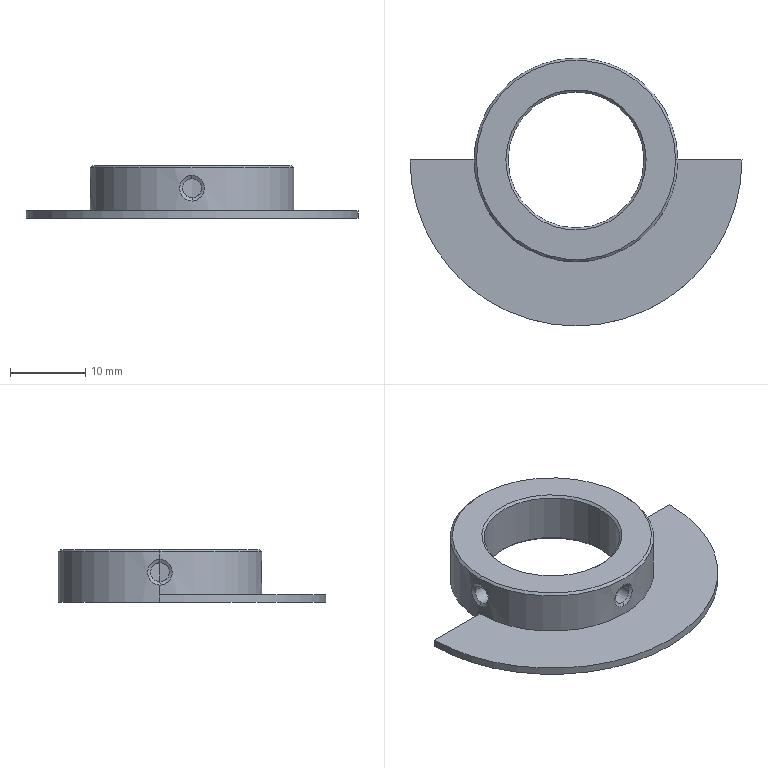Part | NX | 1 solid | 24 faces | box 44 x 35.5 x 7 mm | volume 2646 mm3 | cylinder 9 | cone 6 | plane 5 | spline 4 | commonest cylinder face diameters 2.5 x4 18 x2 27 x2 44 x1
STEP:
#1=CARTESIAN_POINT('',(-13.2,0.,7.));
#2=VERTEX_POINT('',#1);
#3=CARTESIAN_POINT('',(13.2,0.,7.));
#4=VERTEX_POINT('',#3);
#5=CARTESIAN_POINT('',(0.,0.,7.));
#6=DIRECTION('',(0.,0.,-1.));
#7=DIRECTION('',(-1.,0.,0.));
#8=AXIS2_PLACEMENT_3D('',#5,#6,#7);
#9=CIRCLE('',#8,13.2);
#10=EDGE_CURVE('',#2,#4,#9,.T.);
#11=ORIENTED_EDGE('',*,*,#10,.F.);
#12=CARTESIAN_POINT('',(0.,0.,7.));
#13=DIRECTION('',(0.,0.,-1.));
#14=DIRECTION('',(-1.,0.,0.));
#15=AXIS2_PLACEMENT_3D('',#12,#13,#14);
#16=CIRCLE('',#15,13.2);
#17=EDGE_CURVE('',#4,#2,#16,.T.);
#18=ORIENTED_EDGE('',*,*,#17,.F.);
#19=EDGE_LOOP('',(#11,#18));
#20=FACE_BOUND('',#19,.T.);
#21=CARTESIAN_POINT('',(9.3,0.,7.));
#22=VERTEX_POINT('',#21);
#23=CARTESIAN_POINT('',(-9.3,0.,7.));
#24=VERTEX_POINT('',#23);
#25=CARTESIAN_POINT('',(0.,0.,7.));
#26=DIRECTION('',(0.,0.,1.));
#27=DIRECTION('',(1.,0.,0.));
#28=AXIS2_PLACEMENT_3D('',#25,#26,#27);
#29=CIRCLE('',#28,9.3);
#30=EDGE_CURVE('',#22,#24,#29,.T.);
#31=ORIENTED_EDGE('',*,*,#30,.F.);
#32=CARTESIAN_POINT('',(0.,0.,7.));
#33=DIRECTION('',(0.,0.,1.));
#34=DIRECTION('',(1.,0.,0.));
#35=AXIS2_PLACEMENT_3D('',#32,#33,#34);
#36=CIRCLE('',#35,9.3);
#37=EDGE_CURVE('',#24,#22,#36,.T.);
#38=ORIENTED_EDGE('',*,*,#37,.F.);
#39=EDGE_LOOP('',(#31,#38));
#40=FACE_BOUND('',#39,.T.);
#41=CARTESIAN_POINT('',(0.,0.,7.));
#42=DIRECTION('',(0.,0.,1.));
#43=DIRECTION('',(1.,0.,0.));
#44=AXIS2_PLACEMENT_3D('',#41,#42,#43);
#45=PLANE('',#44);
#46=ADVANCED_FACE('',(#20,#40),#45,.T.);
#47=CARTESIAN_POINT('',(13.5,0.,6.7));
#48=VERTEX_POINT('',#47);
#49=CARTESIAN_POINT('',(-13.5,0.,6.7));
#50=VERTEX_POINT('',#49);
#51=CARTESIAN_POINT('',(0.,0.,6.7));
#52=DIRECTION('',(0.,0.,-1.));
#53=DIRECTION('',(-1.,0.,0.));
#54=AXIS2_PLACEMENT_3D('',#51,#52,#53);
#55=CIRCLE('',#54,13.5);
#56=EDGE_CURVE('',#48,#50,#55,.T.);
#57=ORIENTED_EDGE('',*,*,#56,.T.);
#58=CARTESIAN_POINT('',(-13.5,0.,5.7));
#59=VERTEX_POINT('',#58);
#60=CARTESIAN_POINT('',(-13.5,0.,0.));
#61=DIRECTION('',(0.,0.,1.));
#62=VECTOR('',#61,1000.);
#63=LINE('',#60,#62);
#64=EDGE_CURVE('',#50,#59,#63,.F.);
#65=ORIENTED_EDGE('',*,*,#64,.T.);
#66=CARTESIAN_POINT('',(-13.5,-0.01105,2.3));
#67=VERTEX_POINT('',#66);
#68=CARTESIAN_POINT('',(-13.5,0.,5.7));
#69=CARTESIAN_POINT('',(-13.5,-0.4479,5.699));
#70=CARTESIAN_POINT('',(-13.448,-1.303,5.293));
#71=CARTESIAN_POINT('',(-13.378,-1.79,4.006));
#72=CARTESIAN_POINT('',(-13.446,-1.314,2.718));
#73=CARTESIAN_POINT('',(-13.5,-0.4559,2.303));
#74=CARTESIAN_POINT('',(-13.5,-0.01105,2.3));
#75=B_SPLINE_CURVE_WITH_KNOTS('',3,(#68,#69,#70,#71,#72,#73,#74),.UNSPECIFIED.,.F.,.F.,(4,1,1,1,4),(0.,0.25,0.5,0.75,1.),.UNSPECIFIED.);
#76=EDGE_CURVE('',#67,#59,#75,.F.);
#77=ORIENTED_EDGE('',*,*,#76,.F.);
#78=CARTESIAN_POINT('',(-13.5,0.,2.3));
#79=VERTEX_POINT('',#78);
#80=CARTESIAN_POINT('',(-13.5,0.,2.3));
#81=CARTESIAN_POINT('',(-13.5,-0.003678,2.3));
#82=CARTESIAN_POINT('',(-13.5,-0.007364,2.3));
#83=CARTESIAN_POINT('',(-13.5,-0.01105,2.3));
#84=B_SPLINE_CURVE_WITH_KNOTS('',3,(#80,#81,#82,#83),.UNSPECIFIED.,.F.,.F.,(4,4),(9.217,9.227),.UNSPECIFIED.);
#85=EDGE_CURVE('',#79,#67,#84,.T.);
#86=ORIENTED_EDGE('',*,*,#85,.F.);
#87=CARTESIAN_POINT('',(-13.5,0.,1.));
#88=VERTEX_POINT('',#87);
#89=CARTESIAN_POINT('',(-13.5,0.,0.));
#90=DIRECTION('',(0.,0.,1.));
#91=VECTOR('',#90,1000.);
#92=LINE('',#89,#91);
#93=EDGE_CURVE('',#88,#79,#92,.T.);
#94=ORIENTED_EDGE('',*,*,#93,.F.);
#95=CARTESIAN_POINT('',(13.5,0.,1.));
#96=VERTEX_POINT('',#95);
#97=CARTESIAN_POINT('',(0.,0.,1.));
#98=DIRECTION('',(0.,0.,1.));
#99=DIRECTION('',(1.,0.,0.));
#100=AXIS2_PLACEMENT_3D('',#97,#98,#99);
#101=CIRCLE('',#100,13.5);
#102=EDGE_CURVE('',#88,#96,#101,.T.);
#103=ORIENTED_EDGE('',*,*,#102,.T.);
#104=CARTESIAN_POINT('',(13.5,0.,0.));
#105=DIRECTION('',(0.,0.,1.));
#106=VECTOR('',#105,1000.);
#107=LINE('',#104,#106);
#108=EDGE_CURVE('',#48,#96,#107,.F.);
#109=ORIENTED_EDGE('',*,*,#108,.F.);
#110=EDGE_LOOP('',(#57,#65,#77,#86,#94,#103,#109));
#111=FACE_BOUND('',#110,.T.);
#112=CARTESIAN_POINT('',(-0.01314,-13.5,5.7));
#113=VERTEX_POINT('',#112);
#114=CARTESIAN_POINT('',(0.01305,-13.5,2.3));
#115=VERTEX_POINT('',#114);
#116=CARTESIAN_POINT('',(0.01305,-13.5,2.3));
#117=CARTESIAN_POINT('',(-0.4359,-13.5,2.297));
#118=CARTESIAN_POINT('',(-1.296,-13.449,2.698));
#119=CARTESIAN_POINT('',(-1.791,-13.378,3.986));
#120=CARTESIAN_POINT('',(-1.318,-13.446,5.278));
#121=CARTESIAN_POINT('',(-0.4589,-13.5,5.696));
#122=CARTESIAN_POINT('',(-0.01314,-13.5,5.7));
#123=B_SPLINE_CURVE_WITH_KNOTS('',3,(#116,#117,#118,#119,#120,#121,#122),.UNSPECIFIED.,.F.,.F.,(4,1,1,1,4),(0.,0.25,0.5,0.75,1.),.UNSPECIFIED.);
#124=EDGE_CURVE('',#113,#115,#123,.F.);
#125=ORIENTED_EDGE('',*,*,#124,.F.);
#126=CARTESIAN_POINT('',(-0.01314,-13.5,5.7));
#127=CARTESIAN_POINT('',(0.4307,-13.5,5.704));
#128=CARTESIAN_POINT('',(1.299,-13.448,5.302));
#129=CARTESIAN_POINT('',(1.79,-13.378,4.012));
#130=CARTESIAN_POINT('',(1.317,-13.446,2.721));
#131=CARTESIAN_POINT('',(0.4589,-13.5,2.304));
#132=CARTESIAN_POINT('',(0.01305,-13.5,2.3));
#133=B_SPLINE_CURVE_WITH_KNOTS('',3,(#126,#127,#128,#129,#130,#131,#132),.UNSPECIFIED.,.F.,.F.,(4,1,1,1,4),(0.,0.25,0.5,0.75,1.),.UNSPECIFIED.);
#134=EDGE_CURVE('',#115,#113,#133,.F.);
#135=ORIENTED_EDGE('',*,*,#134,.F.);
#136=EDGE_LOOP('',(#125,#135));
#137=FACE_BOUND('',#136,.T.);
#138=CARTESIAN_POINT('',(0.,0.,0.));
#139=DIRECTION('',(0.,0.,1.));
#140=DIRECTION('',(1.,0.,0.));
#141=AXIS2_PLACEMENT_3D('',#138,#139,#140);
#142=CYLINDRICAL_SURFACE('',#141,13.5);
#143=ADVANCED_FACE('',(#111,#137),#142,.T.);
#144=ORIENTED_EDGE('',*,*,#124,.T.);
#145=CARTESIAN_POINT('',(0.009148,-13.24,2.75));
#146=VERTEX_POINT('',#145);
#147=CARTESIAN_POINT('',(0.009148,-13.24,2.75));
#148=CARTESIAN_POINT('',(0.01305,-13.5,2.3));
#149=B_SPLINE_CURVE_WITH_KNOTS('',1,(#147,#148),.UNSPECIFIED.,.F.,.F.,(2,2),(0.,1.),.UNSPECIFIED.);
#150=EDGE_CURVE('',#146,#115,#149,.T.);
#151=ORIENTED_EDGE('',*,*,#150,.F.);
#152=CARTESIAN_POINT('',(-0.0007957,-13.24,2.75));
#153=VERTEX_POINT('',#152);
#154=CARTESIAN_POINT('',(-0.0007956,-13.24,2.75));
#155=CARTESIAN_POINT('',(0.002519,-13.24,2.75));
#156=CARTESIAN_POINT('',(0.005833,-13.24,2.75));
#157=CARTESIAN_POINT('',(0.009147,-13.24,2.75));
#158=B_SPLINE_CURVE_WITH_KNOTS('',3,(#154,#155,#156,#157),.UNSPECIFIED.,.F.,.F.,(4,4),(0.,1.),.UNSPECIFIED.);
#159=EDGE_CURVE('',#153,#146,#158,.T.);
#160=ORIENTED_EDGE('',*,*,#159,.F.);
#161=CARTESIAN_POINT('',(-1.25,-13.182,4.));
#162=VERTEX_POINT('',#161);
#163=CARTESIAN_POINT('',(-1.25,-13.182,4.));
#164=CARTESIAN_POINT('',(-1.25,-13.182,3.841));
#165=CARTESIAN_POINT('',(-1.18,-13.188,3.551));
#166=CARTESIAN_POINT('',(-1.073,-13.198,3.345));
#167=CARTESIAN_POINT('',(-0.8867,-13.211,3.097));
#168=CARTESIAN_POINT('',(-0.6376,-13.225,2.917));
#169=CARTESIAN_POINT('',(-0.4359,-13.234,2.816));
#170=CARTESIAN_POINT('',(-0.1547,-13.24,2.75));
#171=CARTESIAN_POINT('',(-0.0007956,-13.24,2.75));
#172=B_SPLINE_CURVE_WITH_KNOTS('',3,(#163,#164,#165,#166,#167,#168,#169,#170,#171),.UNSPECIFIED.,.F.,.F.,(4,1,1,1,1,1,4),(0.,0.25,0.375,0.5,0.625,0.75,1.),.UNSPECIFIED.);
#173=EDGE_CURVE('',#162,#153,#172,.T.);
#174=ORIENTED_EDGE('',*,*,#173,.F.);
#175=CARTESIAN_POINT('',(-0.009525,-13.24,5.25));
#176=VERTEX_POINT('',#175);
#177=CARTESIAN_POINT('',(-0.009525,-13.24,5.25));
#178=CARTESIAN_POINT('',(-0.1614,-13.24,5.249));
#179=CARTESIAN_POINT('',(-0.4452,-13.234,5.18));
#180=CARTESIAN_POINT('',(-0.6425,-13.225,5.08));
#181=CARTESIAN_POINT('',(-0.891,-13.211,4.899));
#182=CARTESIAN_POINT('',(-1.074,-13.198,4.653));
#183=CARTESIAN_POINT('',(-1.181,-13.188,4.446));
#184=CARTESIAN_POINT('',(-1.25,-13.182,4.158));
#185=CARTESIAN_POINT('',(-1.25,-13.182,4.));
#186=B_SPLINE_CURVE_WITH_KNOTS('',3,(#177,#178,#179,#180,#181,#182,#183,#184,#185),.UNSPECIFIED.,.F.,.F.,(4,1,1,1,1,1,4),(0.,0.25,0.375,0.5,0.625,0.75,1.),.UNSPECIFIED.);
#187=EDGE_CURVE('',#176,#162,#186,.T.);
#188=ORIENTED_EDGE('',*,*,#187,.F.);
#189=CARTESIAN_POINT('',(-0.009525,-13.24,5.25));
#190=CARTESIAN_POINT('',(-0.01314,-13.5,5.7));
#191=B_SPLINE_CURVE_WITH_KNOTS('',1,(#189,#190),.UNSPECIFIED.,.F.,.F.,(2,2),(0.,1.),.UNSPECIFIED.);
#192=EDGE_CURVE('',#176,#113,#191,.T.);
#193=ORIENTED_EDGE('',*,*,#192,.T.);
#194=EDGE_LOOP('',(#144,#151,#160,#174,#188,#193));
#195=FACE_BOUND('',#194,.T.);
#196=CARTESIAN_POINT('',(-0.009525,-13.24,5.25));
#197=CARTESIAN_POINT('',(-0.01314,-13.5,5.7));
#198=CARTESIAN_POINT('',(-0.01524,-13.24,5.25));
#199=CARTESIAN_POINT('',(-0.02103,-13.5,5.7));
#200=CARTESIAN_POINT('',(-0.02096,-13.24,5.25));
#201=CARTESIAN_POINT('',(-0.02892,-13.5,5.7));
#202=CARTESIAN_POINT('',(-0.05049,-13.24,5.249));
#203=CARTESIAN_POINT('',(-0.06965,-13.5,5.699));
#204=CARTESIAN_POINT('',(-0.07427,-13.24,5.248));
#205=CARTESIAN_POINT('',(-0.1025,-13.5,5.697));
#206=CARTESIAN_POINT('',(-0.1973,-13.239,5.238));
#207=CARTESIAN_POINT('',(-0.2718,-13.498,5.682));
#208=CARTESIAN_POINT('',(-0.295,-13.237,5.219));
#209=CARTESIAN_POINT('',(-0.4066,-13.494,5.652));
#210=CARTESIAN_POINT('',(-0.586,-13.229,5.123));
#211=CARTESIAN_POINT('',(-0.7985,-13.479,5.509));
#212=CARTESIAN_POINT('',(-0.7633,-13.219,5.012));
#213=CARTESIAN_POINT('',(-1.031,-13.462,5.344));
#214=CARTESIAN_POINT('',(-1.05,-13.2,4.71));
#215=CARTESIAN_POINT('',(-1.391,-13.429,4.925));
#216=CARTESIAN_POINT('',(-1.154,-13.191,4.524));
#217=CARTESIAN_POINT('',(-1.516,-13.415,4.679));
#218=CARTESIAN_POINT('',(-1.262,-13.181,4.118));
#219=CARTESIAN_POINT('',(-1.644,-13.4,4.15));
#220=CARTESIAN_POINT('',(-1.264,-13.181,3.902));
#221=CARTESIAN_POINT('',(-1.646,-13.399,3.876));
#222=CARTESIAN_POINT('',(-1.162,-13.19,3.492));
#223=CARTESIAN_POINT('',(-1.525,-13.414,3.342));
#224=CARTESIAN_POINT('',(-1.058,-13.199,3.303));
#225=CARTESIAN_POINT('',(-1.402,-13.428,3.092));
#226=CARTESIAN_POINT('',(-0.7739,-13.218,2.996));
#227=CARTESIAN_POINT('',(-1.044,-13.461,2.668));
#228=CARTESIAN_POINT('',(-0.5977,-13.228,2.883));
#229=CARTESIAN_POINT('',(-0.8144,-13.478,2.501));
#230=CARTESIAN_POINT('',(-0.269,-13.238,2.771));
#231=CARTESIAN_POINT('',(-0.3717,-13.496,2.333));
#232=CARTESIAN_POINT('',(-0.1303,-13.24,2.749));
#233=CARTESIAN_POINT('',(-0.1794,-13.5,2.299));
#234=CARTESIAN_POINT('',(0.009148,-13.24,2.75));
#235=CARTESIAN_POINT('',(0.01305,-13.5,2.3));
#236=CARTESIAN_POINT('',(0.009386,-13.24,2.75));
#237=CARTESIAN_POINT('',(0.01338,-13.5,2.3));
#238=CARTESIAN_POINT('',(0.009623,-13.24,2.75));
#239=CARTESIAN_POINT('',(0.01371,-13.5,2.3));
#240=CARTESIAN_POINT('',(0.009861,-13.24,2.75));
#241=CARTESIAN_POINT('',(0.01404,-13.5,2.3));
#242=B_SPLINE_SURFACE_WITH_KNOTS('',3,1,((#196,#197),(#198,#199),(#200,#201),(#202,#203),(#204,#205),(#206,#207),(#208,#209),(#210,#211),(#212,#213),(#214,#215),(#216,#217),(#218,#219),(#220,#221),(#222,#223),(#224,#225),(#226,#227),(#228,#229),(#230,#231),(#232,#233),(#234,#235),(#236,#237),(#238,#239),(#240,#241)),.RULED_SURF.,.F.,.F.,.F.,(4,2,2,2,2,2,2,2,2,3,4),(2,2),(0.,0.02041,0.1054,0.4606,1.192,1.919,2.647,3.381,4.112,4.613,4.614),(0.,1.),.UNSPECIFIED.);
#243=ADVANCED_FACE('',(#195),#242,.F.);
#244=ORIENTED_EDGE('',*,*,#102,.F.);
#245=CARTESIAN_POINT('',(-22.,0.,1.));
#246=VERTEX_POINT('',#245);
#247=CARTESIAN_POINT('',(-22.,0.,1.));
#248=DIRECTION('',(1.,0.,0.));
#249=VECTOR('',#248,1000.);
#250=LINE('',#247,#249);
#251=EDGE_CURVE('',#246,#88,#250,.T.);
#252=ORIENTED_EDGE('',*,*,#251,.F.);
#253=CARTESIAN_POINT('',(22.,0.,1.));
#254=VERTEX_POINT('',#253);
#255=CARTESIAN_POINT('',(0.,0.,1.));
#256=DIRECTION('',(0.,0.,-1.));
#257=DIRECTION('',(1.,0.,0.));
#258=AXIS2_PLACEMENT_3D('',#255,#256,#257);
#259=CIRCLE('',#258,22.);
#260=EDGE_CURVE('',#254,#246,#259,.T.);
#261=ORIENTED_EDGE('',*,*,#260,.F.);
#262=CARTESIAN_POINT('',(13.5,0.,1.));
#263=DIRECTION('',(1.,0.,0.));
#264=VECTOR('',#263,1000.);
#265=LINE('',#262,#264);
#266=EDGE_CURVE('',#96,#254,#265,.T.);
#267=ORIENTED_EDGE('',*,*,#266,.F.);
#268=EDGE_LOOP('',(#244,#252,#261,#267));
#269=FACE_BOUND('',#268,.T.);
#270=CARTESIAN_POINT('',(0.,0.,1.));
#271=DIRECTION('',(0.,0.,1.));
#272=DIRECTION('',(1.,0.,0.));
#273=AXIS2_PLACEMENT_3D('',#270,#271,#272);
#274=PLANE('',#273);
#275=ADVANCED_FACE('',(#269),#274,.T.);
#276=CARTESIAN_POINT('',(13.5,0.,0.));
#277=VERTEX_POINT('',#276);
#278=CARTESIAN_POINT('',(13.5,0.,0.));
#279=DIRECTION('',(0.,0.,1.));
#280=VECTOR('',#279,1000.);
#281=LINE('',#278,#280);
#282=EDGE_CURVE('',#277,#96,#281,.T.);
#283=ORIENTED_EDGE('',*,*,#282,.T.);
#284=ORIENTED_EDGE('',*,*,#266,.T.);
#285=CARTESIAN_POINT('',(22.,0.,0.));
#286=VERTEX_POINT('',#285);
#287=CARTESIAN_POINT('',(22.,0.,0.));
#288=DIRECTION('',(0.,0.,1.));
#289=VECTOR('',#288,1000.);
#290=LINE('',#287,#289);
#291=EDGE_CURVE('',#286,#254,#290,.T.);
#292=ORIENTED_EDGE('',*,*,#291,.F.);
#293=CARTESIAN_POINT('',(0.,0.,0.));
#294=DIRECTION('',(1.,0.,0.));
#295=VECTOR('',#294,1000.);
#296=LINE('',#293,#295);
#297=EDGE_CURVE('',#277,#286,#296,.T.);
#298=ORIENTED_EDGE('',*,*,#297,.F.);
#299=EDGE_LOOP('',(#283,#284,#292,#298));
#300=FACE_BOUND('',#299,.T.);
#301=CARTESIAN_POINT('',(22.,0.,0.));
#302=DIRECTION('',(0.,1.,0.));
#303=DIRECTION('',(1.,0.,0.));
#304=AXIS2_PLACEMENT_3D('',#301,#302,#303);
#305=PLANE('',#304);
#306=ADVANCED_FACE('',(#300),#305,.T.);
#307=CARTESIAN_POINT('',(-13.5,0.,0.));
#308=VERTEX_POINT('',#307);
#309=CARTESIAN_POINT('',(0.,0.,0.));
#310=DIRECTION('',(0.,0.,1.));
#311=DIRECTION('',(1.,0.,0.));
#312=AXIS2_PLACEMENT_3D('',#309,#310,#311);
#313=CIRCLE('',#312,13.5);
#314=EDGE_CURVE('',#277,#308,#313,.T.);
#315=ORIENTED_EDGE('',*,*,#314,.F.);
#316=ORIENTED_EDGE('',*,*,#297,.T.);
#317=CARTESIAN_POINT('',(-22.,0.,0.));
#318=VERTEX_POINT('',#317);
#319=CARTESIAN_POINT('',(0.,0.,0.));
#320=DIRECTION('',(0.,0.,1.));
#321=DIRECTION('',(1.,0.,0.));
#322=AXIS2_PLACEMENT_3D('',#319,#320,#321);
#323=CIRCLE('',#322,22.);
#324=EDGE_CURVE('',#318,#286,#323,.T.);
#325=ORIENTED_EDGE('',*,*,#324,.F.);
#326=CARTESIAN_POINT('',(0.,0.,0.));
#327=DIRECTION('',(1.,0.,0.));
#328=VECTOR('',#327,1000.);
#329=LINE('',#326,#328);
#330=EDGE_CURVE('',#318,#308,#329,.T.);
#331=ORIENTED_EDGE('',*,*,#330,.T.);
#332=EDGE_LOOP('',(#315,#316,#325,#331));
#333=FACE_BOUND('',#332,.T.);
#334=CARTESIAN_POINT('',(9.3,0.,0.));
#335=VERTEX_POINT('',#334);
#336=CARTESIAN_POINT('',(-9.3,0.,0.));
#337=VERTEX_POINT('',#336);
#338=CARTESIAN_POINT('',(0.,0.,0.));
#339=DIRECTION('',(0.,0.,-1.));
#340=DIRECTION('',(-1.,0.,0.));
#341=AXIS2_PLACEMENT_3D('',#338,#339,#340);
#342=CIRCLE('',#341,9.3);
#343=EDGE_CURVE('',#335,#337,#342,.T.);
#344=ORIENTED_EDGE('',*,*,#343,.F.);
#345=CARTESIAN_POINT('',(0.,0.,0.));
#346=DIRECTION('',(0.,0.,-1.));
#347=DIRECTION('',(-1.,0.,0.));
#348=AXIS2_PLACEMENT_3D('',#345,#346,#347);
#349=CIRCLE('',#348,9.3);
#350=EDGE_CURVE('',#337,#335,#349,.T.);
#351=ORIENTED_EDGE('',*,*,#350,.F.);
#352=EDGE_LOOP('',(#344,#351));
#353=FACE_BOUND('',#352,.T.);
#354=CARTESIAN_POINT('',(0.,0.,0.));
#355=DIRECTION('',(0.,0.,1.));
#356=DIRECTION('',(1.,0.,0.));
#357=AXIS2_PLACEMENT_3D('',#354,#355,#356);
#358=PLANE('',#357);
#359=ADVANCED_FACE('',(#333,#353),#358,.F.);
#360=CARTESIAN_POINT('',(-9.,0.,6.7));
#361=VERTEX_POINT('',#360);
#362=CARTESIAN_POINT('',(9.,0.,6.7));
#363=VERTEX_POINT('',#362);
#364=CARTESIAN_POINT('',(0.,0.,6.7));
#365=DIRECTION('',(0.,0.,1.));
#366=DIRECTION('',(1.,0.,0.));
#367=AXIS2_PLACEMENT_3D('',#364,#365,#366);
#368=CIRCLE('',#367,9.);
#369=EDGE_CURVE('',#361,#363,#368,.T.);
#370=ORIENTED_EDGE('',*,*,#369,.T.);
#371=CARTESIAN_POINT('',(9.,0.,0.3));
#372=VERTEX_POINT('',#371);
#373=CARTESIAN_POINT('',(9.,0.,0.));
#374=DIRECTION('',(0.,0.,1.));
#375=VECTOR('',#374,1000.);
#376=LINE('',#373,#375);
#377=EDGE_CURVE('',#363,#372,#376,.F.);
#378=ORIENTED_EDGE('',*,*,#377,.T.);
#379=CARTESIAN_POINT('',(-9.,0.,0.3));
#380=VERTEX_POINT('',#379);
#381=CARTESIAN_POINT('',(0.,0.,0.3));
#382=DIRECTION('',(0.,0.,-1.));
#383=DIRECTION('',(-1.,0.,0.));
#384=AXIS2_PLACEMENT_3D('',#381,#382,#383);
#385=CIRCLE('',#384,9.);
#386=EDGE_CURVE('',#372,#380,#385,.T.);
#387=ORIENTED_EDGE('',*,*,#386,.T.);
#388=CARTESIAN_POINT('',(-9.,0.,2.75));
#389=VERTEX_POINT('',#388);
#390=CARTESIAN_POINT('',(-9.,0.,0.));
#391=DIRECTION('',(0.,0.,1.));
#392=VECTOR('',#391,1000.);
#393=LINE('',#390,#392);
#394=EDGE_CURVE('',#380,#389,#393,.T.);
#395=ORIENTED_EDGE('',*,*,#394,.T.);
#396=CARTESIAN_POINT('',(-8.913,-1.25,4.));
#397=VERTEX_POINT('',#396);
#398=CARTESIAN_POINT('',(-9.,0.,2.75));
#399=CARTESIAN_POINT('',(-9.,-0.6632,2.75));
#400=CARTESIAN_POINT('',(-8.913,-1.249,3.335));
#401=CARTESIAN_POINT('',(-8.913,-1.25,4.));
#402=B_SPLINE_CURVE_WITH_KNOTS('',3,(#398,#399,#400,#401),.UNSPECIFIED.,.F.,.F.,(4,4),(0.,1.),.UNSPECIFIED.);
#403=EDGE_CURVE('',#389,#397,#402,.T.);
#404=ORIENTED_EDGE('',*,*,#403,.T.);
#405=CARTESIAN_POINT('',(-9.,0.,5.25));
#406=VERTEX_POINT('',#405);
#407=CARTESIAN_POINT('',(-8.913,-1.25,4.));
#408=CARTESIAN_POINT('',(-8.913,-1.249,4.664));
#409=CARTESIAN_POINT('',(-9.,-0.6634,5.25));
#410=CARTESIAN_POINT('',(-9.,0.,5.25));
#411=B_SPLINE_CURVE_WITH_KNOTS('',3,(#407,#408,#409,#410),.UNSPECIFIED.,.F.,.F.,(4,4),(0.,1.),.UNSPECIFIED.);
#412=EDGE_CURVE('',#397,#406,#411,.T.);
#413=ORIENTED_EDGE('',*,*,#412,.T.);
#414=CARTESIAN_POINT('',(-9.,0.,0.));
#415=DIRECTION('',(0.,0.,1.));
#416=VECTOR('',#415,1000.);
#417=LINE('',#414,#416);
#418=EDGE_CURVE('',#361,#406,#417,.F.);
#419=ORIENTED_EDGE('',*,*,#418,.F.);
#420=EDGE_LOOP('',(#370,#378,#387,#395,#404,#413,#419));
#421=FACE_BOUND('',#420,.T.);
#422=CARTESIAN_POINT('',(-1.25,-8.913,4.));
#423=VERTEX_POINT('',#422);
#424=CARTESIAN_POINT('',(1.25,-8.913,4.));
#425=VERTEX_POINT('',#424);
#426=CARTESIAN_POINT('',(-1.25,-8.913,4.));
#427=CARTESIAN_POINT('',(-1.25,-8.913,3.668));
#428=CARTESIAN_POINT('',(-0.9792,-8.957,3.023));
#429=CARTESIAN_POINT('',(-0.0001713,-9.022,2.613));
#430=CARTESIAN_POINT('',(0.9799,-8.957,3.024));
#431=CARTESIAN_POINT('',(1.25,-8.913,3.668));
#432=CARTESIAN_POINT('',(1.25,-8.913,4.));
#433=B_SPLINE_CURVE_WITH_KNOTS('',3,(#426,#427,#428,#429,#430,#431,#432),.UNSPECIFIED.,.F.,.F.,(4,1,1,1,4),(0.,0.25,0.5,0.75,1.),.UNSPECIFIED.);
#434=EDGE_CURVE('',#423,#425,#433,.T.);
#435=ORIENTED_EDGE('',*,*,#434,.T.);
#436=CARTESIAN_POINT('',(1.25,-8.913,4.));
#437=CARTESIAN_POINT('',(1.25,-8.913,4.332));
#438=CARTESIAN_POINT('',(0.98,-8.957,4.976));
#439=CARTESIAN_POINT('',(0.0000365,-9.022,5.387));
#440=CARTESIAN_POINT('',(-0.9801,-8.957,4.976));
#441=CARTESIAN_POINT('',(-1.25,-8.913,4.332));
#442=CARTESIAN_POINT('',(-1.25,-8.913,4.));
#443=B_SPLINE_CURVE_WITH_KNOTS('',3,(#436,#437,#438,#439,#440,#441,#442),.UNSPECIFIED.,.F.,.F.,(4,1,1,1,4),(0.,0.25,0.5,0.75,1.),.UNSPECIFIED.);
#444=EDGE_CURVE('',#425,#423,#443,.T.);
#445=ORIENTED_EDGE('',*,*,#444,.T.);
#446=EDGE_LOOP('',(#435,#445));
#447=FACE_BOUND('',#446,.T.);
#448=CARTESIAN_POINT('',(0.,0.,0.));
#449=DIRECTION('',(0.,0.,1.));
#450=DIRECTION('',(1.,0.,0.));
#451=AXIS2_PLACEMENT_3D('',#448,#449,#450);
#452=CYLINDRICAL_SURFACE('',#451,9.);
#453=ADVANCED_FACE('',(#421,#447),#452,.F.);
#454=CARTESIAN_POINT('',(-13.5,0.,0.));
#455=DIRECTION('',(0.,0.,1.));
#456=VECTOR('',#455,1000.);
#457=LINE('',#454,#456);
#458=EDGE_CURVE('',#308,#88,#457,.T.);
#459=ORIENTED_EDGE('',*,*,#458,.F.);
#460=ORIENTED_EDGE('',*,*,#330,.F.);
#461=CARTESIAN_POINT('',(-22.,0.,0.));
#462=DIRECTION('',(0.,0.,1.));
#463=VECTOR('',#462,1000.);
#464=LINE('',#461,#463);
#465=EDGE_CURVE('',#318,#246,#464,.T.);
#466=ORIENTED_EDGE('',*,*,#465,.T.);
#467=ORIENTED_EDGE('',*,*,#251,.T.);
#468=EDGE_LOOP('',(#459,#460,#466,#467));
#469=FACE_BOUND('',#468,.T.);
#470=CARTESIAN_POINT('',(-13.5,0.,0.));
#471=DIRECTION('',(0.,1.,0.));
#472=DIRECTION('',(1.,0.,0.));
#473=AXIS2_PLACEMENT_3D('',#470,#471,#472);
#474=PLANE('',#473);
#475=ADVANCED_FACE('',(#469),#474,.T.);
#476=ORIENTED_EDGE('',*,*,#324,.T.);
#477=ORIENTED_EDGE('',*,*,#291,.T.);
#478=ORIENTED_EDGE('',*,*,#260,.T.);
#479=ORIENTED_EDGE('',*,*,#465,.F.);
#480=EDGE_LOOP('',(#476,#477,#478,#479));
#481=FACE_BOUND('',#480,.T.);
#482=CARTESIAN_POINT('',(0.,0.,0.));
#483=DIRECTION('',(0.,0.,1.));
#484=DIRECTION('',(1.,0.,0.));
#485=AXIS2_PLACEMENT_3D('',#482,#483,#484);
#486=CYLINDRICAL_SURFACE('',#485,22.);
#487=ADVANCED_FACE('',(#481),#486,.T.);
#488=ORIENTED_EDGE('',*,*,#434,.F.);
#489=CARTESIAN_POINT('',(-1.25,-13.5,4.));
#490=DIRECTION('',(0.,-1.,0.));
#491=VECTOR('',#490,1000.);
#492=LINE('',#489,#491);
#493=EDGE_CURVE('',#162,#423,#492,.F.);
#494=ORIENTED_EDGE('',*,*,#493,.F.);
#495=ORIENTED_EDGE('',*,*,#173,.T.);
#496=ORIENTED_EDGE('',*,*,#159,.T.);
#497=CARTESIAN_POINT('',(1.25,-13.182,4.));
#498=VERTEX_POINT('',#497);
#499=CARTESIAN_POINT('',(0.009147,-13.24,2.75));
#500=CARTESIAN_POINT('',(0.1245,-13.24,2.751));
#501=CARTESIAN_POINT('',(0.3981,-13.236,2.779));
#502=CARTESIAN_POINT('',(0.915,-13.211,3.074));
#503=CARTESIAN_POINT('',(1.221,-13.186,3.596));
#504=CARTESIAN_POINT('',(1.25,-13.182,3.879));
#505=CARTESIAN_POINT('',(1.25,-13.182,4.));
#506=B_SPLINE_CURVE_WITH_KNOTS('',3,(#499,#500,#501,#502,#503,#504,#505),.UNSPECIFIED.,.F.,.F.,(4,1,1,1,4),(0.,0.25,0.5,0.75,1.),.UNSPECIFIED.);
#507=EDGE_CURVE('',#146,#498,#506,.T.);
#508=ORIENTED_EDGE('',*,*,#507,.T.);
#509=CARTESIAN_POINT('',(1.25,-13.5,4.));
#510=DIRECTION('',(0.,-1.,0.));
#511=VECTOR('',#510,1000.);
#512=LINE('',#509,#511);
#513=EDGE_CURVE('',#498,#425,#512,.F.);
#514=ORIENTED_EDGE('',*,*,#513,.T.);
#515=EDGE_LOOP('',(#488,#494,#495,#496,#508,#514));
#516=FACE_BOUND('',#515,.T.);
#517=CARTESIAN_POINT('',(0.,-13.5,4.));
#518=DIRECTION('',(0.,-1.,0.));
#519=DIRECTION('',(-1.,0.,0.));
#520=AXIS2_PLACEMENT_3D('',#517,#518,#519);
#521=CYLINDRICAL_SURFACE('',#520,1.25);
#522=ADVANCED_FACE('',(#516),#521,.F.);
#523=CARTESIAN_POINT('',(-13.182,-1.25,4.));
#524=VERTEX_POINT('',#523);
#525=CARTESIAN_POINT('',(-13.24,-0.000798,5.25));
#526=VERTEX_POINT('',#525);
#527=CARTESIAN_POINT('',(-13.182,-1.25,4.));
#528=CARTESIAN_POINT('',(-13.182,-1.25,4.159));
#529=CARTESIAN_POINT('',(-13.188,-1.18,4.449));
#530=CARTESIAN_POINT('',(-13.198,-1.073,4.655));
#531=CARTESIAN_POINT('',(-13.211,-0.8867,4.903));
#532=CARTESIAN_POINT('',(-13.225,-0.6376,5.083));
#533=CARTESIAN_POINT('',(-13.234,-0.4359,5.184));
#534=CARTESIAN_POINT('',(-13.24,-0.1547,5.25));
#535=CARTESIAN_POINT('',(-13.24,-0.000798,5.25));
#536=B_SPLINE_CURVE_WITH_KNOTS('',3,(#527,#528,#529,#530,#531,#532,#533,#534,#535),.UNSPECIFIED.,.F.,.F.,(4,1,1,1,1,1,4),(0.,0.25,0.375,0.5,0.625,0.75,1.),.UNSPECIFIED.);
#537=EDGE_CURVE('',#524,#526,#536,.T.);
#538=ORIENTED_EDGE('',*,*,#537,.T.);
#539=CARTESIAN_POINT('',(-13.24,0.007631,5.25));
#540=VERTEX_POINT('',#539);
#541=CARTESIAN_POINT('',(-13.24,-0.000798,5.25));
#542=CARTESIAN_POINT('',(-13.24,0.002011,5.25));
#543=CARTESIAN_POINT('',(-13.24,0.004821,5.25));
#544=CARTESIAN_POINT('',(-13.24,0.00763,5.25));
#545=B_SPLINE_CURVE_WITH_KNOTS('',3,(#541,#542,#543,#544),.UNSPECIFIED.,.F.,.F.,(4,4),(0.,1.),.UNSPECIFIED.);
#546=EDGE_CURVE('',#526,#540,#545,.T.);
#547=ORIENTED_EDGE('',*,*,#546,.T.);
#548=CARTESIAN_POINT('',(-13.182,1.25,4.));
#549=VERTEX_POINT('',#548);
#550=CARTESIAN_POINT('',(-13.24,0.00763,5.25));
#551=CARTESIAN_POINT('',(-13.24,0.1583,5.249));
#552=CARTESIAN_POINT('',(-13.234,0.4417,5.182));
#553=CARTESIAN_POINT('',(-13.225,0.6422,5.08));
#554=CARTESIAN_POINT('',(-13.211,0.8894,4.9));
#555=CARTESIAN_POINT('',(-13.197,1.076,4.649));
#556=CARTESIAN_POINT('',(-13.188,1.179,4.449));
#557=CARTESIAN_POINT('',(-13.182,1.25,4.158));
#558=CARTESIAN_POINT('',(-13.182,1.25,4.));
#559=B_SPLINE_CURVE_WITH_KNOTS('',3,(#550,#551,#552,#553,#554,#555,#556,#557,#558),.UNSPECIFIED.,.F.,.F.,(4,1,1,1,1,1,4),(0.,0.25,0.375,0.5,0.625,0.75,1.),.UNSPECIFIED.);
#560=EDGE_CURVE('',#540,#549,#559,.T.);
#561=ORIENTED_EDGE('',*,*,#560,.T.);
#562=CARTESIAN_POINT('',(-8.913,1.25,4.));
#563=VERTEX_POINT('',#562);
#564=CARTESIAN_POINT('',(-13.5,1.25,4.));
#565=DIRECTION('',(-1.,0.,0.));
#566=VECTOR('',#565,1000.);
#567=LINE('',#564,#566);
#568=EDGE_CURVE('',#563,#549,#567,.T.);
#569=ORIENTED_EDGE('',*,*,#568,.F.);
#570=CARTESIAN_POINT('',(-8.913,1.25,4.));
#571=CARTESIAN_POINT('',(-8.913,1.25,4.155));
#572=CARTESIAN_POINT('',(-8.922,1.181,4.444));
#573=CARTESIAN_POINT('',(-8.936,1.079,4.644));
#574=CARTESIAN_POINT('',(-8.957,0.8946,4.895));
#575=CARTESIAN_POINT('',(-8.977,0.6463,5.077));
#576=CARTESIAN_POINT('',(-8.991,0.4429,5.182));
#577=CARTESIAN_POINT('',(-9.,0.1549,5.25));
#578=CARTESIAN_POINT('',(-9.,0.,5.25));
#579=B_SPLINE_CURVE_WITH_KNOTS('',3,(#570,#571,#572,#573,#574,#575,#576,#577,#578),.UNSPECIFIED.,.F.,.F.,(4,1,1,1,1,1,4),(0.,0.25,0.375,0.5,0.625,0.75,1.),.UNSPECIFIED.);
#580=EDGE_CURVE('',#406,#563,#579,.F.);
#581=ORIENTED_EDGE('',*,*,#580,.F.);
#582=ORIENTED_EDGE('',*,*,#412,.F.);
#583=CARTESIAN_POINT('',(-13.5,-1.25,4.));
#584=DIRECTION('',(-1.,0.,0.));
#585=VECTOR('',#584,1000.);
#586=LINE('',#583,#585);
#587=EDGE_CURVE('',#397,#524,#586,.T.);
#588=ORIENTED_EDGE('',*,*,#587,.T.);
#589=EDGE_LOOP('',(#538,#547,#561,#569,#581,#582,#588));
#590=FACE_BOUND('',#589,.T.);
#591=CARTESIAN_POINT('',(-13.5,0.,4.));
#592=DIRECTION('',(-1.,0.,0.));
#593=DIRECTION('',(0.,1.,0.));
#594=AXIS2_PLACEMENT_3D('',#591,#592,#593);
#595=CYLINDRICAL_SURFACE('',#594,1.25);
#596=ADVANCED_FACE('',(#590),#595,.F.);
#597=ORIENTED_EDGE('',*,*,#537,.F.);
#598=CARTESIAN_POINT('',(-13.24,-0.008007,2.75));
#599=VERTEX_POINT('',#598);
#600=CARTESIAN_POINT('',(-13.24,-0.008007,2.75));
#601=CARTESIAN_POINT('',(-13.24,-0.1601,2.751));
#602=CARTESIAN_POINT('',(-13.234,-0.4439,2.819));
#603=CARTESIAN_POINT('',(-13.225,-0.6419,2.92));
#604=CARTESIAN_POINT('',(-13.211,-0.8903,3.101));
#605=CARTESIAN_POINT('',(-13.198,-1.073,3.347));
#606=CARTESIAN_POINT('',(-13.188,-1.181,3.553));
#607=CARTESIAN_POINT('',(-13.182,-1.25,3.842));
#608=CARTESIAN_POINT('',(-13.182,-1.25,4.));
#609=B_SPLINE_CURVE_WITH_KNOTS('',3,(#600,#601,#602,#603,#604,#605,#606,#607,#608),.UNSPECIFIED.,.F.,.F.,(4,1,1,1,1,1,4),(0.,0.25,0.375,0.5,0.625,0.75,1.),.UNSPECIFIED.);
#610=EDGE_CURVE('',#599,#524,#609,.T.);
#611=ORIENTED_EDGE('',*,*,#610,.F.);
#612=CARTESIAN_POINT('',(-13.24,-0.008007,2.75));
#613=CARTESIAN_POINT('',(-13.5,-0.01105,2.3));
#614=B_SPLINE_CURVE_WITH_KNOTS('',1,(#612,#613),.UNSPECIFIED.,.F.,.F.,(2,2),(0.,1.),.UNSPECIFIED.);
#615=EDGE_CURVE('',#599,#67,#614,.T.);
#616=ORIENTED_EDGE('',*,*,#615,.T.);
#617=ORIENTED_EDGE('',*,*,#76,.T.);
#618=CARTESIAN_POINT('',(-13.5,0.01096,5.7));
#619=VERTEX_POINT('',#618);
#620=CARTESIAN_POINT('',(-13.5,0.01096,5.7));
#621=CARTESIAN_POINT('',(-13.5,0.007306,5.7));
#622=CARTESIAN_POINT('',(-13.5,0.003653,5.7));
#623=CARTESIAN_POINT('',(-13.5,0.,5.7));
#624=B_SPLINE_CURVE_WITH_KNOTS('',3,(#620,#621,#622,#623),.UNSPECIFIED.,.F.,.F.,(4,4),(0.,1.),.UNSPECIFIED.);
#625=EDGE_CURVE('',#59,#619,#624,.F.);
#626=ORIENTED_EDGE('',*,*,#625,.T.);
#627=CARTESIAN_POINT('',(-13.24,0.007631,5.25));
#628=CARTESIAN_POINT('',(-13.5,0.01096,5.7));
#629=B_SPLINE_CURVE_WITH_KNOTS('',1,(#627,#628),.UNSPECIFIED.,.F.,.F.,(2,2),(0.,1.),.UNSPECIFIED.);
#630=EDGE_CURVE('',#540,#619,#629,.T.);
#631=ORIENTED_EDGE('',*,*,#630,.F.);
#632=ORIENTED_EDGE('',*,*,#546,.F.);
#633=EDGE_LOOP('',(#597,#611,#616,#617,#626,#631,#632));
#634=FACE_BOUND('',#633,.T.);
#635=CARTESIAN_POINT('',(-13.24,-0.008007,2.75));
#636=CARTESIAN_POINT('',(-13.5,-0.01105,2.3));
#637=CARTESIAN_POINT('',(-13.24,-0.01372,2.75));
#638=CARTESIAN_POINT('',(-13.5,-0.01893,2.3));
#639=CARTESIAN_POINT('',(-13.24,-0.01944,2.75));
#640=CARTESIAN_POINT('',(-13.5,-0.02682,2.3));
#641=CARTESIAN_POINT('',(-13.24,-0.04897,2.751));
#642=CARTESIAN_POINT('',(-13.5,-0.06756,2.301));
#643=CARTESIAN_POINT('',(-13.24,-0.07275,2.752));
#644=CARTESIAN_POINT('',(-13.5,-0.1004,2.303));
#645=CARTESIAN_POINT('',(-13.239,-0.1958,2.761));
#646=CARTESIAN_POINT('',(-13.498,-0.2697,2.318));
#647=CARTESIAN_POINT('',(-13.237,-0.2935,2.781));
#648=CARTESIAN_POINT('',(-13.495,-0.4045,2.348));
#649=CARTESIAN_POINT('',(-13.229,-0.5846,2.876));
#650=CARTESIAN_POINT('',(-13.479,-0.7967,2.49));
#651=CARTESIAN_POINT('',(-13.219,-0.7622,2.987));
#652=CARTESIAN_POINT('',(-13.462,-1.029,2.655));
#653=CARTESIAN_POINT('',(-13.2,-1.049,3.289));
#654=CARTESIAN_POINT('',(-13.429,-1.39,3.073));
#655=CARTESIAN_POINT('',(-13.191,-1.154,3.475));
#656=CARTESIAN_POINT('',(-13.415,-1.515,3.319));
#657=CARTESIAN_POINT('',(-13.181,-1.262,3.881));
#658=CARTESIAN_POINT('',(-13.4,-1.644,3.849));
#659=CARTESIAN_POINT('',(-13.181,-1.264,4.097));
#660=CARTESIAN_POINT('',(-13.399,-1.646,4.123));
#661=CARTESIAN_POINT('',(-13.19,-1.162,4.507));
#662=CARTESIAN_POINT('',(-13.414,-1.525,4.657));
#663=CARTESIAN_POINT('',(-13.199,-1.059,4.697));
#664=CARTESIAN_POINT('',(-13.428,-1.402,4.908));
#665=CARTESIAN_POINT('',(-13.218,-0.7742,5.003));
#666=CARTESIAN_POINT('',(-13.461,-1.045,5.332));
#667=CARTESIAN_POINT('',(-13.228,-0.598,5.117));
#668=CARTESIAN_POINT('',(-13.478,-0.8148,5.499));
#669=CARTESIAN_POINT('',(-13.238,-0.2698,5.229));
#670=CARTESIAN_POINT('',(-13.496,-0.3728,5.667));
#671=CARTESIAN_POINT('',(-13.24,-0.1314,5.251));
#672=CARTESIAN_POINT('',(-13.5,-0.181,5.701));
#673=CARTESIAN_POINT('',(-13.24,0.007631,5.25));
#674=CARTESIAN_POINT('',(-13.5,0.01096,5.7));
#675=B_SPLINE_SURFACE_WITH_KNOTS('',3,1,((#635,#636),(#637,#638),(#639,#640),(#641,#642),(#643,#644),(#645,#646),(#647,#648),(#649,#650),(#651,#652),(#653,#654),(#655,#656),(#657,#658),(#659,#660),(#661,#662),(#663,#664),(#665,#666),(#667,#668),(#669,#670),(#671,#672),(#673,#674)),.RULED_SURF.,.F.,.F.,.F.,(4,2,2,2,2,2,2,2,2,4),(2,2),(0.,0.02041,0.1054,0.4605,1.193,1.92,2.648,3.383,4.114,4.613),(0.,1.),.UNSPECIFIED.);
#676=ADVANCED_FACE('',(#634),#675,.F.);
#677=ORIENTED_EDGE('',*,*,#56,.F.);
#678=CARTESIAN_POINT('',(13.5,0.,6.7));
#679=DIRECTION('',(0.7071,0.,-0.7071));
#680=VECTOR('',#679,1000.);
#681=LINE('',#678,#680);
#682=EDGE_CURVE('',#4,#48,#681,.T.);
#683=ORIENTED_EDGE('',*,*,#682,.F.);
#684=ORIENTED_EDGE('',*,*,#17,.T.);
#685=CARTESIAN_POINT('',(-13.5,0.,6.7));
#686=DIRECTION('',(-0.7071,0.,-0.7071));
#687=VECTOR('',#686,1000.);
#688=LINE('',#685,#687);
#689=EDGE_CURVE('',#2,#50,#688,.T.);
#690=ORIENTED_EDGE('',*,*,#689,.T.);
#691=EDGE_LOOP('',(#677,#683,#684,#690));
#692=FACE_BOUND('',#691,.T.);
#693=CARTESIAN_POINT('',(0.,0.,6.7));
#694=DIRECTION('',(0.,0.,-1.));
#695=DIRECTION('',(-1.,0.,0.));
#696=AXIS2_PLACEMENT_3D('',#693,#694,#695);
#697=CONICAL_SURFACE('',#696,13.5,0.7854);
#698=ADVANCED_FACE('',(#692),#697,.T.);
#699=ORIENTED_EDGE('',*,*,#30,.T.);
#700=CARTESIAN_POINT('',(-9.3,0.,7.));
#701=DIRECTION('',(-0.7071,0.,0.7071));
#702=VECTOR('',#701,1000.);
#703=LINE('',#700,#702);
#704=EDGE_CURVE('',#24,#361,#703,.F.);
#705=ORIENTED_EDGE('',*,*,#704,.T.);
#706=CARTESIAN_POINT('',(0.,0.,6.7));
#707=DIRECTION('',(0.,0.,1.));
#708=DIRECTION('',(1.,0.,0.));
#709=AXIS2_PLACEMENT_3D('',#706,#707,#708);
#710=CIRCLE('',#709,9.);
#711=EDGE_CURVE('',#363,#361,#710,.T.);
#712=ORIENTED_EDGE('',*,*,#711,.F.);
#713=CARTESIAN_POINT('',(9.3,0.,7.));
#714=DIRECTION('',(0.7071,0.,0.7071));
#715=VECTOR('',#714,1000.);
#716=LINE('',#713,#715);
#717=EDGE_CURVE('',#22,#363,#716,.F.);
#718=ORIENTED_EDGE('',*,*,#717,.F.);
#719=EDGE_LOOP('',(#699,#705,#712,#718));
#720=FACE_BOUND('',#719,.T.);
#721=CARTESIAN_POINT('',(0.,0.,7.));
#722=DIRECTION('',(0.,0.,1.));
#723=DIRECTION('',(1.,0.,0.));
#724=AXIS2_PLACEMENT_3D('',#721,#722,#723);
#725=CONICAL_SURFACE('',#724,9.3,0.7854);
#726=ADVANCED_FACE('',(#720),#725,.F.);
#727=ORIENTED_EDGE('',*,*,#343,.T.);
#728=CARTESIAN_POINT('',(-9.3,0.,0.));
#729=DIRECTION('',(-0.7071,0.,-0.7071));
#730=VECTOR('',#729,1000.);
#731=LINE('',#728,#730);
#732=EDGE_CURVE('',#337,#380,#731,.F.);
#733=ORIENTED_EDGE('',*,*,#732,.T.);
#734=ORIENTED_EDGE('',*,*,#386,.F.);
#735=CARTESIAN_POINT('',(9.3,0.,0.));
#736=DIRECTION('',(0.7071,0.,-0.7071));
#737=VECTOR('',#736,1000.);
#738=LINE('',#735,#737);
#739=EDGE_CURVE('',#335,#372,#738,.F.);
#740=ORIENTED_EDGE('',*,*,#739,.F.);
#741=EDGE_LOOP('',(#727,#733,#734,#740));
#742=FACE_BOUND('',#741,.T.);
#743=CARTESIAN_POINT('',(0.,0.,0.));
#744=DIRECTION('',(0.,0.,-1.));
#745=DIRECTION('',(-1.,0.,0.));
#746=AXIS2_PLACEMENT_3D('',#743,#744,#745);
#747=CONICAL_SURFACE('',#746,9.3,0.7854);
#748=ADVANCED_FACE('',(#742),#747,.F.);
#749=CARTESIAN_POINT('',(-8.913,1.25,4.));
#750=CARTESIAN_POINT('',(-8.913,1.249,3.336));
#751=CARTESIAN_POINT('',(-9.,0.6635,2.75));
#752=CARTESIAN_POINT('',(-9.,0.,2.75));
#753=B_SPLINE_CURVE_WITH_KNOTS('',3,(#749,#750,#751,#752),.UNSPECIFIED.,.F.,.F.,(4,4),(0.,1.),.UNSPECIFIED.);
#754=EDGE_CURVE('',#563,#389,#753,.T.);
#755=ORIENTED_EDGE('',*,*,#754,.T.);
#756=ORIENTED_EDGE('',*,*,#394,.F.);
#757=CARTESIAN_POINT('',(0.,0.,0.3));
#758=DIRECTION('',(0.,0.,-1.));
#759=DIRECTION('',(-1.,0.,0.));
#760=AXIS2_PLACEMENT_3D('',#757,#758,#759);
#761=CIRCLE('',#760,9.);
#762=EDGE_CURVE('',#380,#372,#761,.T.);
#763=ORIENTED_EDGE('',*,*,#762,.T.);
#764=ORIENTED_EDGE('',*,*,#377,.F.);
#765=ORIENTED_EDGE('',*,*,#711,.T.);
#766=ORIENTED_EDGE('',*,*,#418,.T.);
#767=ORIENTED_EDGE('',*,*,#580,.T.);
#768=EDGE_LOOP('',(#755,#756,#763,#764,#765,#766,#767));
#769=FACE_BOUND('',#768,.T.);
#770=CARTESIAN_POINT('',(0.,0.,0.));
#771=DIRECTION('',(0.,0.,1.));
#772=DIRECTION('',(1.,0.,0.));
#773=AXIS2_PLACEMENT_3D('',#770,#771,#772);
#774=CYLINDRICAL_SURFACE('',#773,9.);
#775=ADVANCED_FACE('',(#769),#774,.F.);
#776=ORIENTED_EDGE('',*,*,#369,.F.);
#777=ORIENTED_EDGE('',*,*,#704,.F.);
#778=ORIENTED_EDGE('',*,*,#37,.T.);
#779=ORIENTED_EDGE('',*,*,#717,.T.);
#780=EDGE_LOOP('',(#776,#777,#778,#779));
#781=FACE_BOUND('',#780,.T.);
#782=CARTESIAN_POINT('',(0.,0.,7.));
#783=DIRECTION('',(0.,0.,1.));
#784=DIRECTION('',(1.,0.,0.));
#785=AXIS2_PLACEMENT_3D('',#782,#783,#784);
#786=CONICAL_SURFACE('',#785,9.3,0.7854);
#787=ADVANCED_FACE('',(#781),#786,.F.);
#788=ORIENTED_EDGE('',*,*,#568,.T.);
#789=CARTESIAN_POINT('',(-13.182,1.25,4.));
#790=CARTESIAN_POINT('',(-13.182,1.25,3.845));
#791=CARTESIAN_POINT('',(-13.189,1.179,3.547));
#792=CARTESIAN_POINT('',(-13.198,1.072,3.345));
#793=CARTESIAN_POINT('',(-13.212,0.8837,3.094));
#794=CARTESIAN_POINT('',(-13.225,0.6324,2.914));
#795=CARTESIAN_POINT('',(-13.234,0.4295,2.813));
#796=CARTESIAN_POINT('',(-13.24,0.1435,2.749));
#797=CARTESIAN_POINT('',(-13.24,-0.008007,2.75));
#798=B_SPLINE_CURVE_WITH_KNOTS('',3,(#789,#790,#791,#792,#793,#794,#795,#796,#797),.UNSPECIFIED.,.F.,.F.,(4,1,1,1,1,1,4),(0.,0.25,0.375,0.5,0.625,0.75,1.),.UNSPECIFIED.);
#799=EDGE_CURVE('',#549,#599,#798,.T.);
#800=ORIENTED_EDGE('',*,*,#799,.T.);
#801=ORIENTED_EDGE('',*,*,#610,.T.);
#802=ORIENTED_EDGE('',*,*,#587,.F.);
#803=ORIENTED_EDGE('',*,*,#403,.F.);
#804=ORIENTED_EDGE('',*,*,#754,.F.);
#805=EDGE_LOOP('',(#788,#800,#801,#802,#803,#804));
#806=FACE_BOUND('',#805,.T.);
#807=CARTESIAN_POINT('',(-13.5,0.,4.));
#808=DIRECTION('',(-1.,0.,0.));
#809=DIRECTION('',(0.,1.,0.));
#810=AXIS2_PLACEMENT_3D('',#807,#808,#809);
#811=CYLINDRICAL_SURFACE('',#810,1.25);
#812=ADVANCED_FACE('',(#806),#811,.F.);
#813=ORIENTED_EDGE('',*,*,#10,.T.);
#814=ORIENTED_EDGE('',*,*,#682,.T.);
#815=CARTESIAN_POINT('',(0.,0.,6.7));
#816=DIRECTION('',(0.,0.,-1.));
#817=DIRECTION('',(-1.,0.,0.));
#818=AXIS2_PLACEMENT_3D('',#815,#816,#817);
#819=CIRCLE('',#818,13.5);
#820=EDGE_CURVE('',#50,#48,#819,.T.);
#821=ORIENTED_EDGE('',*,*,#820,.F.);
#822=ORIENTED_EDGE('',*,*,#689,.F.);
#823=EDGE_LOOP('',(#813,#814,#821,#822));
#824=FACE_BOUND('',#823,.T.);
#825=CARTESIAN_POINT('',(0.,0.,6.7));
#826=DIRECTION('',(0.,0.,-1.));
#827=DIRECTION('',(-1.,0.,0.));
#828=AXIS2_PLACEMENT_3D('',#825,#826,#827);
#829=CONICAL_SURFACE('',#828,13.5,0.7854);
#830=ADVANCED_FACE('',(#824),#829,.T.);
#831=ORIENTED_EDGE('',*,*,#732,.F.);
#832=ORIENTED_EDGE('',*,*,#350,.T.);
#833=ORIENTED_EDGE('',*,*,#739,.T.);
#834=ORIENTED_EDGE('',*,*,#762,.F.);
#835=EDGE_LOOP('',(#831,#832,#833,#834));
#836=FACE_BOUND('',#835,.T.);
#837=CARTESIAN_POINT('',(0.,0.,0.));
#838=DIRECTION('',(0.,0.,-1.));
#839=DIRECTION('',(-1.,0.,0.));
#840=AXIS2_PLACEMENT_3D('',#837,#838,#839);
#841=CONICAL_SURFACE('',#840,9.3,0.7854);
#842=ADVANCED_FACE('',(#836),#841,.F.);
#843=ORIENTED_EDGE('',*,*,#493,.T.);
#844=ORIENTED_EDGE('',*,*,#444,.F.);
#845=ORIENTED_EDGE('',*,*,#513,.F.);
#846=CARTESIAN_POINT('',(1.25,-13.182,4.));
#847=CARTESIAN_POINT('',(1.25,-13.182,4.155));
#848=CARTESIAN_POINT('',(1.178,-13.189,4.454));
#849=CARTESIAN_POINT('',(1.072,-13.198,4.655));
#850=CARTESIAN_POINT('',(0.8831,-13.212,4.907));
#851=CARTESIAN_POINT('',(0.6317,-13.225,5.086));
#852=CARTESIAN_POINT('',(0.4282,-13.234,5.187));
#853=CARTESIAN_POINT('',(0.1421,-13.24,5.251));
#854=CARTESIAN_POINT('',(-0.009525,-13.24,5.25));
#855=B_SPLINE_CURVE_WITH_KNOTS('',3,(#846,#847,#848,#849,#850,#851,#852,#853,#854),.UNSPECIFIED.,.F.,.F.,(4,1,1,1,1,1,4),(0.,0.25,0.375,0.5,0.625,0.75,1.),.UNSPECIFIED.);
#856=EDGE_CURVE('',#498,#176,#855,.T.);
#857=ORIENTED_EDGE('',*,*,#856,.T.);
#858=ORIENTED_EDGE('',*,*,#187,.T.);
#859=EDGE_LOOP('',(#843,#844,#845,#857,#858));
#860=FACE_BOUND('',#859,.T.);
#861=CARTESIAN_POINT('',(0.,-13.5,4.));
#862=DIRECTION('',(0.,-1.,0.));
#863=DIRECTION('',(-1.,0.,0.));
#864=AXIS2_PLACEMENT_3D('',#861,#862,#863);
#865=CYLINDRICAL_SURFACE('',#864,1.25);
#866=ADVANCED_FACE('',(#860),#865,.F.);
#867=ORIENTED_EDGE('',*,*,#625,.F.);
#868=ORIENTED_EDGE('',*,*,#64,.F.);
#869=ORIENTED_EDGE('',*,*,#820,.T.);
#870=ORIENTED_EDGE('',*,*,#108,.T.);
#871=ORIENTED_EDGE('',*,*,#282,.F.);
#872=ORIENTED_EDGE('',*,*,#314,.T.);
#873=ORIENTED_EDGE('',*,*,#458,.T.);
#874=ORIENTED_EDGE('',*,*,#93,.T.);
#875=CARTESIAN_POINT('',(-13.5,0.,2.3));
#876=CARTESIAN_POINT('',(-13.5,0.4417,2.3));
#877=CARTESIAN_POINT('',(-13.448,1.306,2.707));
#878=CARTESIAN_POINT('',(-13.378,1.79,3.996));
#879=CARTESIAN_POINT('',(-13.447,1.313,5.283));
#880=CARTESIAN_POINT('',(-13.5,0.4559,5.697));
#881=CARTESIAN_POINT('',(-13.5,0.01096,5.7));
#882=B_SPLINE_CURVE_WITH_KNOTS('',3,(#875,#876,#877,#878,#879,#880,#881),.UNSPECIFIED.,.F.,.F.,(4,1,1,1,4),(0.,0.25,0.5,0.75,1.),.UNSPECIFIED.);
#883=EDGE_CURVE('',#619,#79,#882,.F.);
#884=ORIENTED_EDGE('',*,*,#883,.F.);
#885=EDGE_LOOP('',(#867,#868,#869,#870,#871,#872,#873,#874,#884));
#886=FACE_BOUND('',#885,.T.);
#887=CARTESIAN_POINT('',(0.,0.,0.));
#888=DIRECTION('',(0.,0.,1.));
#889=DIRECTION('',(1.,0.,0.));
#890=AXIS2_PLACEMENT_3D('',#887,#888,#889);
#891=CYLINDRICAL_SURFACE('',#890,13.5);
#892=ADVANCED_FACE('',(#886),#891,.T.);
#893=ORIENTED_EDGE('',*,*,#630,.T.);
#894=ORIENTED_EDGE('',*,*,#883,.T.);
#895=ORIENTED_EDGE('',*,*,#85,.T.);
#896=ORIENTED_EDGE('',*,*,#615,.F.);
#897=ORIENTED_EDGE('',*,*,#799,.F.);
#898=ORIENTED_EDGE('',*,*,#560,.F.);
#899=EDGE_LOOP('',(#893,#894,#895,#896,#897,#898));
#900=FACE_BOUND('',#899,.T.);
#901=CARTESIAN_POINT('',(-13.24,0.007631,5.25));
#902=CARTESIAN_POINT('',(-13.5,0.01096,5.7));
#903=CARTESIAN_POINT('',(-13.24,0.07081,5.25));
#904=CARTESIAN_POINT('',(-13.5,0.09817,5.699));
#905=CARTESIAN_POINT('',(-13.24,0.1341,5.244));
#906=CARTESIAN_POINT('',(-13.499,0.1854,5.691));
#907=CARTESIAN_POINT('',(-13.236,0.3995,5.202));
#908=CARTESIAN_POINT('',(-13.492,0.5481,5.627));
#909=CARTESIAN_POINT('',(-13.228,0.5904,5.121));
#910=CARTESIAN_POINT('',(-13.478,0.8058,5.503));
#911=CARTESIAN_POINT('',(-13.209,0.9214,4.87));
#912=CARTESIAN_POINT('',(-13.445,1.232,5.145));
#913=CARTESIAN_POINT('',(-13.199,1.055,4.703));
#914=CARTESIAN_POINT('',(-13.428,1.396,4.917));
#915=CARTESIAN_POINT('',(-13.185,1.227,4.319));
#916=CARTESIAN_POINT('',(-13.405,1.603,4.409));
#917=CARTESIAN_POINT('',(-13.181,1.263,4.106));
#918=CARTESIAN_POINT('',(-13.399,1.645,4.138));
#919=CARTESIAN_POINT('',(-13.184,1.228,3.685));
#920=CARTESIAN_POINT('',(-13.404,1.604,3.593));
#921=CARTESIAN_POINT('',(-13.191,1.157,3.482));
#922=CARTESIAN_POINT('',(-13.415,1.52,3.331));
#923=CARTESIAN_POINT('',(-13.209,0.9249,3.134));
#924=CARTESIAN_POINT('',(-13.444,1.235,2.86));
#925=CARTESIAN_POINT('',(-13.219,0.7682,2.993));
#926=CARTESIAN_POINT('',(-13.462,1.037,2.66));
#927=CARTESIAN_POINT('',(-13.235,0.4044,2.799));
#928=CARTESIAN_POINT('',(-13.491,0.5573,2.378));
#929=CARTESIAN_POINT('',(-13.24,0.2042,2.75));
#930=CARTESIAN_POINT('',(-13.5,0.281,2.3));
#931=CARTESIAN_POINT('',(-13.24,-0.002655,2.75));
#932=CARTESIAN_POINT('',(-13.5,-0.003654,2.3));
#933=CARTESIAN_POINT('',(-13.24,-0.005329,2.75));
#934=CARTESIAN_POINT('',(-13.5,-0.007353,2.3));
#935=CARTESIAN_POINT('',(-13.24,-0.008007,2.75));
#936=CARTESIAN_POINT('',(-13.5,-0.01105,2.3));
#937=B_SPLINE_SURFACE_WITH_KNOTS('',3,1,((#901,#902),(#903,#904),(#905,#906),(#907,#908),(#909,#910),(#911,#912),(#913,#914),(#915,#916),(#917,#918),(#919,#920),(#921,#922),(#923,#924),(#925,#926),(#927,#928),(#929,#930),(#931,#932),(#933,#934),(#935,#936)),.RULED_SURF.,.F.,.F.,.F.,(4,2,2,2,2,2,2,2,4),(2,2),(4.613,4.841,5.569,6.303,7.031,7.761,8.49,9.217,9.227),(0.,1.),.UNSPECIFIED.);
#938=ADVANCED_FACE('',(#900),#937,.F.);
#939=ORIENTED_EDGE('',*,*,#150,.T.);
#940=ORIENTED_EDGE('',*,*,#134,.T.);
#941=ORIENTED_EDGE('',*,*,#192,.F.);
#942=ORIENTED_EDGE('',*,*,#856,.F.);
#943=ORIENTED_EDGE('',*,*,#507,.F.);
#944=EDGE_LOOP('',(#939,#940,#941,#942,#943));
#945=FACE_BOUND('',#944,.T.);
#946=CARTESIAN_POINT('',(0.009148,-13.24,2.75));
#947=CARTESIAN_POINT('',(0.01305,-13.5,2.3));
#948=CARTESIAN_POINT('',(0.07196,-13.24,2.75));
#949=CARTESIAN_POINT('',(0.09975,-13.5,2.301));
#950=CARTESIAN_POINT('',(0.1349,-13.24,2.756));
#951=CARTESIAN_POINT('',(0.1865,-13.499,2.309));
#952=CARTESIAN_POINT('',(0.3998,-13.236,2.798));
#953=CARTESIAN_POINT('',(0.5485,-13.492,2.373));
#954=CARTESIAN_POINT('',(0.5907,-13.228,2.879));
#955=CARTESIAN_POINT('',(0.8061,-13.478,2.497));
#956=CARTESIAN_POINT('',(0.9215,-13.209,3.13));
#957=CARTESIAN_POINT('',(1.233,-13.445,2.855));
#958=CARTESIAN_POINT('',(1.055,-13.199,3.297));
#959=CARTESIAN_POINT('',(1.396,-13.428,3.083));
#960=CARTESIAN_POINT('',(1.227,-13.185,3.681));
#961=CARTESIAN_POINT('',(1.603,-13.405,3.591));
#962=CARTESIAN_POINT('',(1.263,-13.181,3.894));
#963=CARTESIAN_POINT('',(1.645,-13.399,3.862));
#964=CARTESIAN_POINT('',(1.228,-13.184,4.314));
#965=CARTESIAN_POINT('',(1.604,-13.404,4.406));
#966=CARTESIAN_POINT('',(1.157,-13.191,4.518));
#967=CARTESIAN_POINT('',(1.521,-13.415,4.669));
#968=CARTESIAN_POINT('',(0.925,-13.209,4.866));
#969=CARTESIAN_POINT('',(1.235,-13.444,5.14));
#970=CARTESIAN_POINT('',(0.7682,-13.219,5.007));
#971=CARTESIAN_POINT('',(1.037,-13.462,5.34));
#972=CARTESIAN_POINT('',(0.4042,-13.235,5.201));
#973=CARTESIAN_POINT('',(0.5571,-13.491,5.622));
#974=CARTESIAN_POINT('',(0.2041,-13.24,5.25));
#975=CARTESIAN_POINT('',(0.2808,-13.5,5.7));
#976=CARTESIAN_POINT('',(-0.003196,-13.24,5.25));
#977=CARTESIAN_POINT('',(-0.004398,-13.5,5.7));
#978=CARTESIAN_POINT('',(-0.006359,-13.24,5.25));
#979=CARTESIAN_POINT('',(-0.008773,-13.5,5.7));
#980=CARTESIAN_POINT('',(-0.009525,-13.24,5.25));
#981=CARTESIAN_POINT('',(-0.01314,-13.5,5.7));
#982=B_SPLINE_SURFACE_WITH_KNOTS('',3,1,((#946,#947),(#948,#949),(#950,#951),(#952,#953),(#954,#955),(#956,#957),(#958,#959),(#960,#961),(#962,#963),(#964,#965),(#966,#967),(#968,#969),(#970,#971),(#972,#973),(#974,#975),(#976,#977),(#978,#979),(#980,#981)),.RULED_SURF.,.F.,.F.,.F.,(4,2,2,2,2,2,2,2,4),(2,2),(4.613,4.839,5.568,6.302,7.029,7.759,8.489,9.216,9.227),(0.,1.),.UNSPECIFIED.);
#983=ADVANCED_FACE('',(#945),#982,.F.);
#984=CLOSED_SHELL('',(#46,#143,#243,#275,#306,#359,#453,#475,#487,#522,#596,#676,#698,#726,#748,#775,#787,#812,#830,#842,#866,#892,#938,#983));
#985=MANIFOLD_SOLID_BREP('',#984);
#986=(LENGTH_UNIT()NAMED_UNIT(*)SI_UNIT(.MILLI.,.METRE.));
#987=UNCERTAINTY_MEASURE_WITH_UNIT(LENGTH_MEASURE(0.0508),#986,'','');
#988=(NAMED_UNIT(*)PLANE_ANGLE_UNIT()SI_UNIT($,.RADIAN.));
#989=(NAMED_UNIT(*)SI_UNIT($,.STERADIAN.)SOLID_ANGLE_UNIT());
#990=(GEOMETRIC_REPRESENTATION_CONTEXT(3)GLOBAL_UNCERTAINTY_ASSIGNED_CONTEXT((#987))GLOBAL_UNIT_ASSIGNED_CONTEXT((#986,#988,#989))REPRESENTATION_CONTEXT('',''));
#991=ADVANCED_BREP_SHAPE_REPRESENTATION('',(#985),#990);